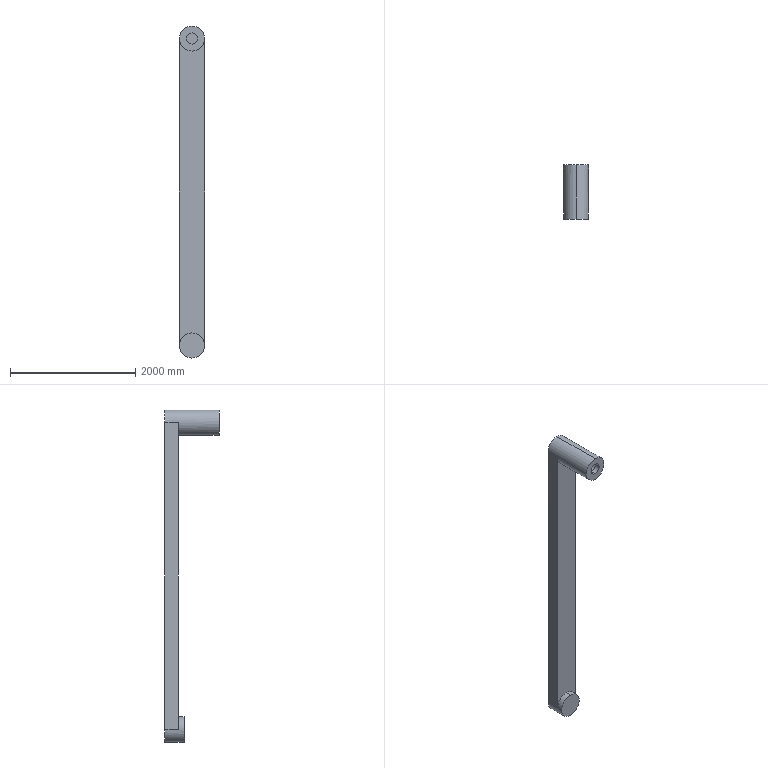Part | SolidWorks | features ICE 5, Extrusion 1 | 1 solid | 19 faces | box 400 x 866 x 5303 mm | volume 491224658 mm3 | cylinder 10 | plane 9 | commonest cylinder face diameters 400 x4 180 x2 250 x2 275 x2
STEP:
#1=CARTESIAN_POINT('',(0.,-176.,5040.555));
#2=VERTEX_POINT('',#1);
#3=CARTESIAN_POINT('',(0.,-176.,4765.555));
#4=VERTEX_POINT('',#3);
#5=CARTESIAN_POINT('',(0.,-176.,4903.055));
#6=DIRECTION('',(0.,-1.,0.));
#7=DIRECTION('',(0.,0.,-1.));
#8=AXIS2_PLACEMENT_3D('',#5,#6,#7);
#9=CIRCLE('',#8,137.5);
#10=EDGE_CURVE('',#2,#4,#9,.T.);
#11=ORIENTED_EDGE('',*,*,#10,.F.);
#12=CARTESIAN_POINT('',(0.,-780.,5040.555));
#13=VERTEX_POINT('',#12);
#14=CARTESIAN_POINT('',(0.,-176.,5040.555));
#15=DIRECTION('',(0.,-1.,0.));
#16=VECTOR('',#15,1000.);
#17=LINE('',#14,#16);
#18=EDGE_CURVE('',#2,#13,#17,.T.);
#19=ORIENTED_EDGE('',*,*,#18,.T.);
#20=CARTESIAN_POINT('',(0.,-780.,4765.555));
#21=VERTEX_POINT('',#20);
#22=CARTESIAN_POINT('',(0.,-780.,4903.055));
#23=DIRECTION('',(0.,1.,0.));
#24=DIRECTION('',(0.,0.,-1.));
#25=AXIS2_PLACEMENT_3D('',#22,#23,#24);
#26=CIRCLE('',#25,137.5);
#27=EDGE_CURVE('',#21,#13,#26,.T.);
#28=ORIENTED_EDGE('',*,*,#27,.F.);
#29=CARTESIAN_POINT('',(0.,-176.,4765.555));
#30=DIRECTION('',(0.,-1.,0.));
#31=VECTOR('',#30,1000.);
#32=LINE('',#29,#31);
#33=EDGE_CURVE('',#4,#21,#32,.T.);
#34=ORIENTED_EDGE('',*,*,#33,.F.);
#35=EDGE_LOOP('',(#11,#19,#28,#34));
#36=FACE_OUTER_BOUND('',#35,.T.);
#37=CARTESIAN_POINT('',(0.,-176.,4903.055));
#38=DIRECTION('',(0.,-1.,0.));
#39=DIRECTION('',(0.,0.,-1.));
#40=AXIS2_PLACEMENT_3D('',#37,#38,#39);
#41=CYLINDRICAL_SURFACE('',#40,137.5);
#42=ADVANCED_FACE('',(#36),#41,.F.);
#43=CARTESIAN_POINT('',(0.,-866.,4993.055));
#44=VERTEX_POINT('',#43);
#45=CARTESIAN_POINT('',(0.,-866.,4813.055));
#46=VERTEX_POINT('',#45);
#47=CARTESIAN_POINT('',(0.,-866.,4903.055));
#48=DIRECTION('',(0.,-1.,0.));
#49=DIRECTION('',(0.,0.,-1.));
#50=AXIS2_PLACEMENT_3D('',#47,#48,#49);
#51=CIRCLE('',#50,90.);
#52=EDGE_CURVE('',#44,#46,#51,.T.);
#53=ORIENTED_EDGE('',*,*,#52,.T.);
#54=CARTESIAN_POINT('',(0.,-780.,4813.055));
#55=VERTEX_POINT('',#54);
#56=CARTESIAN_POINT('',(0.,-866.,4813.055));
#57=DIRECTION('',(0.,1.,0.));
#58=VECTOR('',#57,1000.);
#59=LINE('',#56,#58);
#60=EDGE_CURVE('',#46,#55,#59,.T.);
#61=ORIENTED_EDGE('',*,*,#60,.T.);
#62=CARTESIAN_POINT('',(0.,-780.,4993.055));
#63=VERTEX_POINT('',#62);
#64=CARTESIAN_POINT('',(0.,-780.,4903.055));
#65=DIRECTION('',(0.,-1.,0.));
#66=DIRECTION('',(0.,0.,-1.));
#67=AXIS2_PLACEMENT_3D('',#64,#65,#66);
#68=CIRCLE('',#67,90.);
#69=EDGE_CURVE('',#63,#55,#68,.T.);
#70=ORIENTED_EDGE('',*,*,#69,.F.);
#71=CARTESIAN_POINT('',(0.,-866.,4993.055));
#72=DIRECTION('',(0.,1.,0.));
#73=VECTOR('',#72,1000.);
#74=LINE('',#71,#73);
#75=EDGE_CURVE('',#44,#63,#74,.T.);
#76=ORIENTED_EDGE('',*,*,#75,.F.);
#77=EDGE_LOOP('',(#53,#61,#70,#76));
#78=FACE_OUTER_BOUND('',#77,.T.);
#79=CARTESIAN_POINT('',(0.,-866.,4903.055));
#80=DIRECTION('',(0.,1.,0.));
#81=DIRECTION('',(0.,0.,1.));
#82=AXIS2_PLACEMENT_3D('',#79,#80,#81);
#83=CYLINDRICAL_SURFACE('',#82,90.);
#84=ADVANCED_FACE('',(#78),#83,.F.);
#85=CARTESIAN_POINT('',(0.,-866.,4703.055));
#86=VERTEX_POINT('',#85);
#87=CARTESIAN_POINT('',(0.,-866.,5103.055));
#88=VERTEX_POINT('',#87);
#89=CARTESIAN_POINT('',(0.,-866.,4903.055));
#90=DIRECTION('',(0.,-1.,0.));
#91=DIRECTION('',(0.,0.,-1.));
#92=AXIS2_PLACEMENT_3D('',#89,#90,#91);
#93=CIRCLE('',#92,200.);
#94=EDGE_CURVE('',#86,#88,#93,.T.);
#95=ORIENTED_EDGE('',*,*,#94,.F.);
#96=CARTESIAN_POINT('',(0.,-214.,4703.055));
#97=VERTEX_POINT('',#96);
#98=CARTESIAN_POINT('',(0.,-780.,4703.055));
#99=DIRECTION('',(0.,1.,0.));
#100=VECTOR('',#99,1000.);
#101=LINE('',#98,#100);
#102=EDGE_CURVE('',#86,#97,#101,.T.);
#103=ORIENTED_EDGE('',*,*,#102,.T.);
#104=CARTESIAN_POINT('',(200.,-214.,4903.055));
#105=VERTEX_POINT('',#104);
#106=CARTESIAN_POINT('',(0.,-214.,4903.055));
#107=DIRECTION('',(0.,1.,0.));
#108=DIRECTION('',(0.,0.,1.));
#109=AXIS2_PLACEMENT_3D('',#106,#107,#108);
#110=CIRCLE('',#109,200.);
#111=EDGE_CURVE('',#105,#97,#110,.T.);
#112=ORIENTED_EDGE('',*,*,#111,.F.);
#113=CARTESIAN_POINT('',(200.,0.,4903.055));
#114=VERTEX_POINT('',#113);
#115=CARTESIAN_POINT('',(200.,-214.,4903.055));
#116=DIRECTION('',(0.,1.,0.));
#117=VECTOR('',#116,1000.);
#118=LINE('',#115,#117);
#119=EDGE_CURVE('',#105,#114,#118,.T.);
#120=ORIENTED_EDGE('',*,*,#119,.T.);
#121=CARTESIAN_POINT('',(0.,0.,5103.055));
#122=VERTEX_POINT('',#121);
#123=CARTESIAN_POINT('',(0.,0.,4903.055));
#124=DIRECTION('',(0.,1.,0.));
#125=DIRECTION('',(0.,0.,1.));
#126=AXIS2_PLACEMENT_3D('',#123,#124,#125);
#127=CIRCLE('',#126,200.);
#128=EDGE_CURVE('',#122,#114,#127,.T.);
#129=ORIENTED_EDGE('',*,*,#128,.F.);
#130=CARTESIAN_POINT('',(0.,-780.,5103.055));
#131=DIRECTION('',(0.,1.,0.));
#132=VECTOR('',#131,1000.);
#133=LINE('',#130,#132);
#134=EDGE_CURVE('',#88,#122,#133,.T.);
#135=ORIENTED_EDGE('',*,*,#134,.F.);
#136=EDGE_LOOP('',(#95,#103,#112,#120,#129,#135));
#137=FACE_OUTER_BOUND('',#136,.T.);
#138=CARTESIAN_POINT('',(0.,-780.,4903.055));
#139=DIRECTION('',(0.,1.,0.));
#140=DIRECTION('',(0.,0.,1.));
#141=AXIS2_PLACEMENT_3D('',#138,#139,#140);
#142=CYLINDRICAL_SURFACE('',#141,200.);
#143=ADVANCED_FACE('',(#137),#142,.T.);
#144=CARTESIAN_POINT('',(0.,-220.,-125.));
#145=VERTEX_POINT('',#144);
#146=CARTESIAN_POINT('',(0.,-220.,125.));
#147=VERTEX_POINT('',#146);
#148=CARTESIAN_POINT('',(0.,-220.,0.));
#149=DIRECTION('',(0.,1.,0.));
#150=DIRECTION('',(0.,0.,1.));
#151=AXIS2_PLACEMENT_3D('',#148,#149,#150);
#152=CIRCLE('',#151,125.);
#153=EDGE_CURVE('',#145,#147,#152,.T.);
#154=ORIENTED_EDGE('',*,*,#153,.F.);
#155=CARTESIAN_POINT('',(0.,0.,-125.));
#156=VERTEX_POINT('',#155);
#157=CARTESIAN_POINT('',(0.,-220.,-125.));
#158=DIRECTION('',(0.,1.,0.));
#159=VECTOR('',#158,1000.);
#160=LINE('',#157,#159);
#161=EDGE_CURVE('',#145,#156,#160,.T.);
#162=ORIENTED_EDGE('',*,*,#161,.T.);
#163=CARTESIAN_POINT('',(0.,0.,125.));
#164=VERTEX_POINT('',#163);
#165=CARTESIAN_POINT('',(0.,0.,0.));
#166=DIRECTION('',(0.,1.,0.));
#167=DIRECTION('',(0.,0.,1.));
#168=AXIS2_PLACEMENT_3D('',#165,#166,#167);
#169=CIRCLE('',#168,125.);
#170=EDGE_CURVE('',#156,#164,#169,.T.);
#171=ORIENTED_EDGE('',*,*,#170,.T.);
#172=CARTESIAN_POINT('',(0.,-220.,125.));
#173=DIRECTION('',(0.,1.,0.));
#174=VECTOR('',#173,1000.);
#175=LINE('',#172,#174);
#176=EDGE_CURVE('',#147,#164,#175,.T.);
#177=ORIENTED_EDGE('',*,*,#176,.F.);
#178=EDGE_LOOP('',(#154,#162,#171,#177));
#179=FACE_OUTER_BOUND('',#178,.T.);
#180=CARTESIAN_POINT('',(0.,-220.,0.));
#181=DIRECTION('',(0.,1.,0.));
#182=DIRECTION('',(0.,0.,1.));
#183=AXIS2_PLACEMENT_3D('',#180,#181,#182);
#184=CYLINDRICAL_SURFACE('',#183,125.);
#185=ADVANCED_FACE('',(#179),#184,.F.);
#186=CARTESIAN_POINT('',(0.,-306.,-200.));
#187=VERTEX_POINT('',#186);
#188=CARTESIAN_POINT('',(0.,-306.,200.));
#189=VERTEX_POINT('',#188);
#190=CARTESIAN_POINT('',(0.,-306.,0.));
#191=DIRECTION('',(0.,-1.,0.));
#192=DIRECTION('',(0.,0.,-1.));
#193=AXIS2_PLACEMENT_3D('',#190,#191,#192);
#194=CIRCLE('',#193,200.);
#195=EDGE_CURVE('',#187,#189,#194,.T.);
#196=ORIENTED_EDGE('',*,*,#195,.F.);
#197=CARTESIAN_POINT('',(0.,0.,-200.));
#198=VERTEX_POINT('',#197);
#199=CARTESIAN_POINT('',(0.,-220.,-200.));
#200=DIRECTION('',(0.,1.,0.));
#201=VECTOR('',#200,1000.);
#202=LINE('',#199,#201);
#203=EDGE_CURVE('',#187,#198,#202,.T.);
#204=ORIENTED_EDGE('',*,*,#203,.T.);
#205=CARTESIAN_POINT('',(200.,0.,0.));
#206=VERTEX_POINT('',#205);
#207=CARTESIAN_POINT('',(0.,0.,0.));
#208=DIRECTION('',(0.,1.,0.));
#209=DIRECTION('',(0.,0.,1.));
#210=AXIS2_PLACEMENT_3D('',#207,#208,#209);
#211=CIRCLE('',#210,200.);
#212=EDGE_CURVE('',#206,#198,#211,.T.);
#213=ORIENTED_EDGE('',*,*,#212,.F.);
#214=CARTESIAN_POINT('',(200.,-214.,0.));
#215=VERTEX_POINT('',#214);
#216=CARTESIAN_POINT('',(200.,-214.,0.));
#217=DIRECTION('',(0.,1.,0.));
#218=VECTOR('',#217,1000.);
#219=LINE('',#216,#218);
#220=EDGE_CURVE('',#215,#206,#219,.T.);
#221=ORIENTED_EDGE('',*,*,#220,.F.);
#222=CARTESIAN_POINT('',(0.,-214.,200.));
#223=VERTEX_POINT('',#222);
#224=CARTESIAN_POINT('',(0.,-214.,0.));
#225=DIRECTION('',(0.,1.,0.));
#226=DIRECTION('',(0.,0.,1.));
#227=AXIS2_PLACEMENT_3D('',#224,#225,#226);
#228=CIRCLE('',#227,200.);
#229=EDGE_CURVE('',#223,#215,#228,.T.);
#230=ORIENTED_EDGE('',*,*,#229,.F.);
#231=CARTESIAN_POINT('',(0.,-220.,200.));
#232=DIRECTION('',(0.,1.,0.));
#233=VECTOR('',#232,1000.);
#234=LINE('',#231,#233);
#235=EDGE_CURVE('',#189,#223,#234,.T.);
#236=ORIENTED_EDGE('',*,*,#235,.F.);
#237=EDGE_LOOP('',(#196,#204,#213,#221,#230,#236));
#238=FACE_OUTER_BOUND('',#237,.T.);
#239=CARTESIAN_POINT('',(0.,-220.,0.));
#240=DIRECTION('',(0.,1.,0.));
#241=DIRECTION('',(0.,0.,1.));
#242=AXIS2_PLACEMENT_3D('',#239,#240,#241);
#243=CYLINDRICAL_SURFACE('',#242,200.);
#244=ADVANCED_FACE('',(#238),#243,.T.);
#245=ORIENTED_EDGE('',*,*,#203,.F.);
#246=CARTESIAN_POINT('',(0.,-306.,0.));
#247=DIRECTION('',(0.,-1.,0.));
#248=DIRECTION('',(0.,0.,-1.));
#249=AXIS2_PLACEMENT_3D('',#246,#247,#248);
#250=CIRCLE('',#249,200.);
#251=EDGE_CURVE('',#189,#187,#250,.T.);
#252=ORIENTED_EDGE('',*,*,#251,.F.);
#253=ORIENTED_EDGE('',*,*,#235,.T.);
#254=CARTESIAN_POINT('',(-200.,-214.,0.));
#255=VERTEX_POINT('',#254);
#256=CARTESIAN_POINT('',(0.,-214.,0.));
#257=DIRECTION('',(0.,1.,0.));
#258=DIRECTION('',(0.,0.,1.));
#259=AXIS2_PLACEMENT_3D('',#256,#257,#258);
#260=CIRCLE('',#259,200.);
#261=EDGE_CURVE('',#255,#223,#260,.T.);
#262=ORIENTED_EDGE('',*,*,#261,.F.);
#263=CARTESIAN_POINT('',(-200.,0.,0.));
#264=VERTEX_POINT('',#263);
#265=CARTESIAN_POINT('',(-200.,-214.,0.));
#266=DIRECTION('',(0.,1.,0.));
#267=VECTOR('',#266,1000.);
#268=LINE('',#265,#267);
#269=EDGE_CURVE('',#255,#264,#268,.T.);
#270=ORIENTED_EDGE('',*,*,#269,.T.);
#271=CARTESIAN_POINT('',(0.,0.,0.));
#272=DIRECTION('',(0.,1.,0.));
#273=DIRECTION('',(0.,0.,1.));
#274=AXIS2_PLACEMENT_3D('',#271,#272,#273);
#275=CIRCLE('',#274,200.);
#276=EDGE_CURVE('',#198,#264,#275,.T.);
#277=ORIENTED_EDGE('',*,*,#276,.F.);
#278=EDGE_LOOP('',(#245,#252,#253,#262,#270,#277));
#279=FACE_OUTER_BOUND('',#278,.T.);
#280=CARTESIAN_POINT('',(0.,-220.,0.));
#281=DIRECTION('',(0.,1.,0.));
#282=DIRECTION('',(0.,0.,1.));
#283=AXIS2_PLACEMENT_3D('',#280,#281,#282);
#284=CYLINDRICAL_SURFACE('',#283,200.);
#285=ADVANCED_FACE('',(#279),#284,.T.);
#286=CARTESIAN_POINT('',(0.,0.,0.));
#287=DIRECTION('',(0.,1.,0.));
#288=DIRECTION('',(0.,0.,1.));
#289=AXIS2_PLACEMENT_3D('',#286,#287,#288);
#290=CIRCLE('',#289,125.);
#291=EDGE_CURVE('',#164,#156,#290,.T.);
#292=ORIENTED_EDGE('',*,*,#291,.F.);
#293=ORIENTED_EDGE('',*,*,#170,.F.);
#294=EDGE_LOOP('',(#292,#293));
#295=FACE_BOUND('',#294,.T.);
#296=ORIENTED_EDGE('',*,*,#212,.T.);
#297=ORIENTED_EDGE('',*,*,#276,.T.);
#298=CARTESIAN_POINT('',(-200.,0.,4903.055));
#299=VERTEX_POINT('',#298);
#300=CARTESIAN_POINT('',(-200.,0.,0.));
#301=DIRECTION('',(0.,0.,1.));
#302=VECTOR('',#301,1000.);
#303=LINE('',#300,#302);
#304=EDGE_CURVE('',#264,#299,#303,.T.);
#305=ORIENTED_EDGE('',*,*,#304,.T.);
#306=CARTESIAN_POINT('',(0.,0.,4903.055));
#307=DIRECTION('',(0.,1.,0.));
#308=DIRECTION('',(0.,0.,1.));
#309=AXIS2_PLACEMENT_3D('',#306,#307,#308);
#310=CIRCLE('',#309,200.);
#311=EDGE_CURVE('',#299,#122,#310,.T.);
#312=ORIENTED_EDGE('',*,*,#311,.T.);
#313=ORIENTED_EDGE('',*,*,#128,.T.);
#314=CARTESIAN_POINT('',(200.,0.,0.));
#315=DIRECTION('',(0.,0.,1.));
#316=VECTOR('',#315,1000.);
#317=LINE('',#314,#316);
#318=EDGE_CURVE('',#206,#114,#317,.T.);
#319=ORIENTED_EDGE('',*,*,#318,.F.);
#320=EDGE_LOOP('',(#296,#297,#305,#312,#313,#319));
#321=FACE_OUTER_BOUND('',#320,.T.);
#322=CARTESIAN_POINT('',(0.,0.,0.));
#323=DIRECTION('',(0.,1.,0.));
#324=DIRECTION('',(0.,0.,1.));
#325=AXIS2_PLACEMENT_3D('',#322,#323,#324);
#326=PLANE('',#325);
#327=ADVANCED_FACE('',(#295,#321),#326,.T.);
#328=ORIENTED_EDGE('',*,*,#161,.F.);
#329=CARTESIAN_POINT('',(0.,-220.,0.));
#330=DIRECTION('',(0.,1.,0.));
#331=DIRECTION('',(0.,0.,1.));
#332=AXIS2_PLACEMENT_3D('',#329,#330,#331);
#333=CIRCLE('',#332,125.);
#334=EDGE_CURVE('',#147,#145,#333,.T.);
#335=ORIENTED_EDGE('',*,*,#334,.F.);
#336=ORIENTED_EDGE('',*,*,#176,.T.);
#337=ORIENTED_EDGE('',*,*,#291,.T.);
#338=EDGE_LOOP('',(#328,#335,#336,#337));
#339=FACE_OUTER_BOUND('',#338,.T.);
#340=CARTESIAN_POINT('',(0.,-220.,0.));
#341=DIRECTION('',(0.,1.,0.));
#342=DIRECTION('',(0.,0.,1.));
#343=AXIS2_PLACEMENT_3D('',#340,#341,#342);
#344=CYLINDRICAL_SURFACE('',#343,125.);
#345=ADVANCED_FACE('',(#339),#344,.F.);
#346=ORIENTED_EDGE('',*,*,#318,.T.);
#347=ORIENTED_EDGE('',*,*,#119,.F.);
#348=CARTESIAN_POINT('',(200.,-214.,0.));
#349=DIRECTION('',(0.,0.,1.));
#350=VECTOR('',#349,1000.);
#351=LINE('',#348,#350);
#352=EDGE_CURVE('',#215,#105,#351,.T.);
#353=ORIENTED_EDGE('',*,*,#352,.F.);
#354=ORIENTED_EDGE('',*,*,#220,.T.);
#355=EDGE_LOOP('',(#346,#347,#353,#354));
#356=FACE_OUTER_BOUND('',#355,.T.);
#357=CARTESIAN_POINT('',(200.,-214.,0.));
#358=DIRECTION('',(-1.,0.,0.));
#359=DIRECTION('',(0.,0.,1.));
#360=AXIS2_PLACEMENT_3D('',#357,#358,#359);
#361=PLANE('',#360);
#362=ADVANCED_FACE('',(#356),#361,.F.);
#363=ORIENTED_EDGE('',*,*,#304,.F.);
#364=ORIENTED_EDGE('',*,*,#269,.F.);
#365=CARTESIAN_POINT('',(-200.,-214.,4903.055));
#366=VERTEX_POINT('',#365);
#367=CARTESIAN_POINT('',(-200.,-214.,0.));
#368=DIRECTION('',(0.,0.,1.));
#369=VECTOR('',#368,1000.);
#370=LINE('',#367,#369);
#371=EDGE_CURVE('',#255,#366,#370,.T.);
#372=ORIENTED_EDGE('',*,*,#371,.T.);
#373=CARTESIAN_POINT('',(-200.,-214.,4903.055));
#374=DIRECTION('',(0.,1.,0.));
#375=VECTOR('',#374,1000.);
#376=LINE('',#373,#375);
#377=EDGE_CURVE('',#366,#299,#376,.T.);
#378=ORIENTED_EDGE('',*,*,#377,.T.);
#379=EDGE_LOOP('',(#363,#364,#372,#378));
#380=FACE_OUTER_BOUND('',#379,.T.);
#381=CARTESIAN_POINT('',(-200.,-214.,0.));
#382=DIRECTION('',(-1.,0.,0.));
#383=DIRECTION('',(0.,0.,1.));
#384=AXIS2_PLACEMENT_3D('',#381,#382,#383);
#385=PLANE('',#384);
#386=ADVANCED_FACE('',(#380),#385,.T.);
#387=ORIENTED_EDGE('',*,*,#261,.T.);
#388=ORIENTED_EDGE('',*,*,#229,.T.);
#389=ORIENTED_EDGE('',*,*,#352,.T.);
#390=ORIENTED_EDGE('',*,*,#111,.T.);
#391=CARTESIAN_POINT('',(0.,-214.,4903.055));
#392=DIRECTION('',(0.,1.,0.));
#393=DIRECTION('',(0.,0.,1.));
#394=AXIS2_PLACEMENT_3D('',#391,#392,#393);
#395=CIRCLE('',#394,200.);
#396=EDGE_CURVE('',#97,#366,#395,.T.);
#397=ORIENTED_EDGE('',*,*,#396,.T.);
#398=ORIENTED_EDGE('',*,*,#371,.F.);
#399=EDGE_LOOP('',(#387,#388,#389,#390,#397,#398));
#400=FACE_OUTER_BOUND('',#399,.T.);
#401=CARTESIAN_POINT('',(0.,-214.,0.));
#402=DIRECTION('',(0.,1.,0.));
#403=DIRECTION('',(0.,0.,1.));
#404=AXIS2_PLACEMENT_3D('',#401,#402,#403);
#405=PLANE('',#404);
#406=ADVANCED_FACE('',(#400),#405,.F.);
#407=ORIENTED_EDGE('',*,*,#102,.F.);
#408=CARTESIAN_POINT('',(0.,-866.,4903.055));
#409=DIRECTION('',(0.,-1.,0.));
#410=DIRECTION('',(0.,0.,-1.));
#411=AXIS2_PLACEMENT_3D('',#408,#409,#410);
#412=CIRCLE('',#411,200.);
#413=EDGE_CURVE('',#88,#86,#412,.T.);
#414=ORIENTED_EDGE('',*,*,#413,.F.);
#415=ORIENTED_EDGE('',*,*,#134,.T.);
#416=ORIENTED_EDGE('',*,*,#311,.F.);
#417=ORIENTED_EDGE('',*,*,#377,.F.);
#418=ORIENTED_EDGE('',*,*,#396,.F.);
#419=EDGE_LOOP('',(#407,#414,#415,#416,#417,#418));
#420=FACE_OUTER_BOUND('',#419,.T.);
#421=CARTESIAN_POINT('',(0.,-780.,4903.055));
#422=DIRECTION('',(0.,1.,0.));
#423=DIRECTION('',(0.,0.,1.));
#424=AXIS2_PLACEMENT_3D('',#421,#422,#423);
#425=CYLINDRICAL_SURFACE('',#424,200.);
#426=ADVANCED_FACE('',(#420),#425,.T.);
#427=ORIENTED_EDGE('',*,*,#69,.T.);
#428=CARTESIAN_POINT('',(0.,-780.,4903.055));
#429=DIRECTION('',(0.,-1.,0.));
#430=DIRECTION('',(0.,0.,-1.));
#431=AXIS2_PLACEMENT_3D('',#428,#429,#430);
#432=CIRCLE('',#431,90.);
#433=EDGE_CURVE('',#55,#63,#432,.T.);
#434=ORIENTED_EDGE('',*,*,#433,.T.);
#435=EDGE_LOOP('',(#427,#434));
#436=FACE_BOUND('',#435,.T.);
#437=ORIENTED_EDGE('',*,*,#27,.T.);
#438=CARTESIAN_POINT('',(0.,-780.,4903.055));
#439=DIRECTION('',(0.,1.,0.));
#440=DIRECTION('',(0.,0.,-1.));
#441=AXIS2_PLACEMENT_3D('',#438,#439,#440);
#442=CIRCLE('',#441,137.5);
#443=EDGE_CURVE('',#13,#21,#442,.T.);
#444=ORIENTED_EDGE('',*,*,#443,.T.);
#445=EDGE_LOOP('',(#437,#444));
#446=FACE_OUTER_BOUND('',#445,.T.);
#447=CARTESIAN_POINT('',(0.,-780.,4903.055));
#448=DIRECTION('',(0.,-1.,0.));
#449=DIRECTION('',(0.,0.,-1.));
#450=AXIS2_PLACEMENT_3D('',#447,#448,#449);
#451=PLANE('',#450);
#452=ADVANCED_FACE('',(#436,#446),#451,.F.);
#453=ORIENTED_EDGE('',*,*,#413,.T.);
#454=ORIENTED_EDGE('',*,*,#94,.T.);
#455=EDGE_LOOP('',(#453,#454));
#456=FACE_OUTER_BOUND('',#455,.T.);
#457=ORIENTED_EDGE('',*,*,#52,.F.);
#458=CARTESIAN_POINT('',(0.,-866.,4903.055));
#459=DIRECTION('',(0.,-1.,0.));
#460=DIRECTION('',(0.,0.,-1.));
#461=AXIS2_PLACEMENT_3D('',#458,#459,#460);
#462=CIRCLE('',#461,90.);
#463=EDGE_CURVE('',#46,#44,#462,.T.);
#464=ORIENTED_EDGE('',*,*,#463,.F.);
#465=EDGE_LOOP('',(#457,#464));
#466=FACE_BOUND('',#465,.T.);
#467=CARTESIAN_POINT('',(0.,-866.,4903.055));
#468=DIRECTION('',(0.,-1.,0.));
#469=DIRECTION('',(0.,0.,-1.));
#470=AXIS2_PLACEMENT_3D('',#467,#468,#469);
#471=PLANE('',#470);
#472=ADVANCED_FACE('',(#456,#466),#471,.T.);
#473=ORIENTED_EDGE('',*,*,#60,.F.);
#474=ORIENTED_EDGE('',*,*,#463,.T.);
#475=ORIENTED_EDGE('',*,*,#75,.T.);
#476=ORIENTED_EDGE('',*,*,#433,.F.);
#477=EDGE_LOOP('',(#473,#474,#475,#476));
#478=FACE_OUTER_BOUND('',#477,.T.);
#479=CARTESIAN_POINT('',(0.,-866.,4903.055));
#480=DIRECTION('',(0.,1.,0.));
#481=DIRECTION('',(0.,0.,1.));
#482=AXIS2_PLACEMENT_3D('',#479,#480,#481);
#483=CYLINDRICAL_SURFACE('',#482,90.);
#484=ADVANCED_FACE('',(#478),#483,.F.);
#485=CARTESIAN_POINT('',(0.,-176.,4903.055));
#486=DIRECTION('',(0.,-1.,0.));
#487=DIRECTION('',(0.,0.,-1.));
#488=AXIS2_PLACEMENT_3D('',#485,#486,#487);
#489=CIRCLE('',#488,137.5);
#490=EDGE_CURVE('',#4,#2,#489,.T.);
#491=ORIENTED_EDGE('',*,*,#490,.T.);
#492=ORIENTED_EDGE('',*,*,#10,.T.);
#493=EDGE_LOOP('',(#491,#492));
#494=FACE_OUTER_BOUND('',#493,.T.);
#495=CARTESIAN_POINT('',(0.,-176.,4903.055));
#496=DIRECTION('',(0.,-1.,0.));
#497=DIRECTION('',(0.,0.,-1.));
#498=AXIS2_PLACEMENT_3D('',#495,#496,#497);
#499=PLANE('',#498);
#500=ADVANCED_FACE('',(#494),#499,.T.);
#501=ORIENTED_EDGE('',*,*,#18,.F.);
#502=ORIENTED_EDGE('',*,*,#490,.F.);
#503=ORIENTED_EDGE('',*,*,#33,.T.);
#504=ORIENTED_EDGE('',*,*,#443,.F.);
#505=EDGE_LOOP('',(#501,#502,#503,#504));
#506=FACE_OUTER_BOUND('',#505,.T.);
#507=CARTESIAN_POINT('',(0.,-176.,4903.055));
#508=DIRECTION('',(0.,-1.,0.));
#509=DIRECTION('',(0.,0.,-1.));
#510=AXIS2_PLACEMENT_3D('',#507,#508,#509);
#511=CYLINDRICAL_SURFACE('',#510,137.5);
#512=ADVANCED_FACE('',(#506),#511,.F.);
#513=ORIENTED_EDGE('',*,*,#334,.T.);
#514=ORIENTED_EDGE('',*,*,#153,.T.);
#515=EDGE_LOOP('',(#513,#514));
#516=FACE_OUTER_BOUND('',#515,.T.);
#517=CARTESIAN_POINT('',(0.,-220.,0.));
#518=DIRECTION('',(0.,-1.,0.));
#519=DIRECTION('',(0.,0.,-1.));
#520=AXIS2_PLACEMENT_3D('',#517,#518,#519);
#521=PLANE('',#520);
#522=ADVANCED_FACE('',(#516),#521,.F.);
#523=ORIENTED_EDGE('',*,*,#251,.T.);
#524=ORIENTED_EDGE('',*,*,#195,.T.);
#525=EDGE_LOOP('',(#523,#524));
#526=FACE_OUTER_BOUND('',#525,.T.);
#527=CARTESIAN_POINT('',(0.,-306.,0.));
#528=DIRECTION('',(0.,-1.,0.));
#529=DIRECTION('',(0.,0.,-1.));
#530=AXIS2_PLACEMENT_3D('',#527,#528,#529);
#531=PLANE('',#530);
#532=ADVANCED_FACE('',(#526),#531,.T.);
#533=CLOSED_SHELL('',(#42,#84,#143,#185,#244,#285,#327,#345,#362,#386,#406,#426,#452,#472,#484,#500,#512,#522,#532));
#534=MANIFOLD_SOLID_BREP('',#533);
#535=CARTESIAN_POINT('',(0.,0.,0.));
#536=DIRECTION('',(0.,0.,1.));
#537=DIRECTION('',(1.,0.,0.));
#538=AXIS2_PLACEMENT_3D('',#535,#536,#537);
#539=(LENGTH_UNIT()NAMED_UNIT(*)SI_UNIT(.MILLI.,.METRE.));
#540=UNCERTAINTY_MEASURE_WITH_UNIT(LENGTH_MEASURE(0.00001),#539,'','');
#541=(NAMED_UNIT(*)PLANE_ANGLE_UNIT()SI_UNIT($,.RADIAN.));
#542=(NAMED_UNIT(*)SI_UNIT($,.STERADIAN.)SOLID_ANGLE_UNIT());
#543=(GEOMETRIC_REPRESENTATION_CONTEXT(3)GLOBAL_UNCERTAINTY_ASSIGNED_CONTEXT((#540))GLOBAL_UNIT_ASSIGNED_CONTEXT((#539,#541,#542))REPRESENTATION_CONTEXT('',''));
#544=ADVANCED_BREP_SHAPE_REPRESENTATION('',(#534,#538),#543);